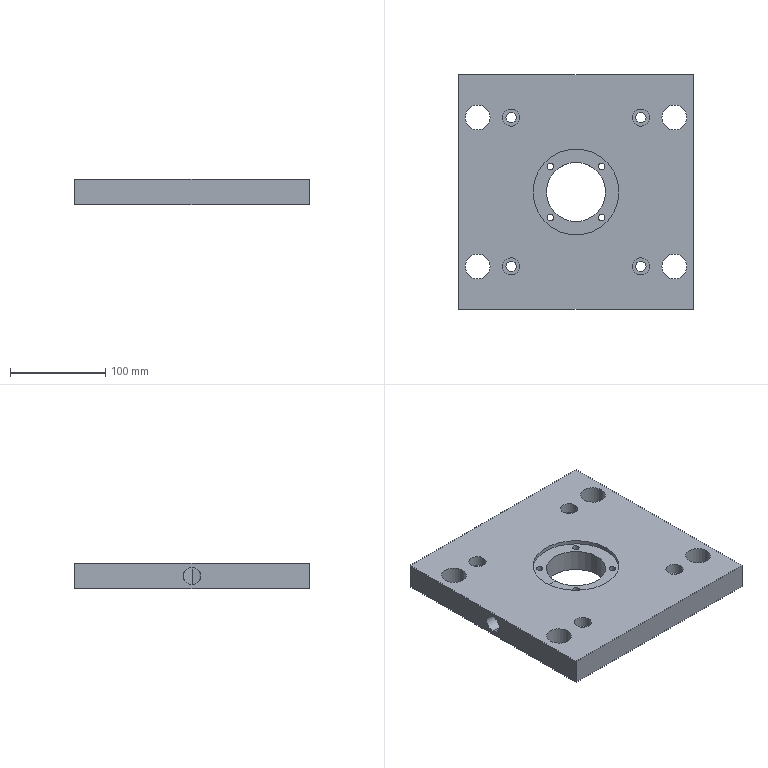Part | STEP file | 1 | 1 solid | 49 faces | box 246 x 246 x 27 mm | volume 1437591 mm3 | cylinder 38 | plane 11 | commonest cylinder face diameters 18 x10 6.8 x8 11 x8 26 x8 62 x2 90 x2